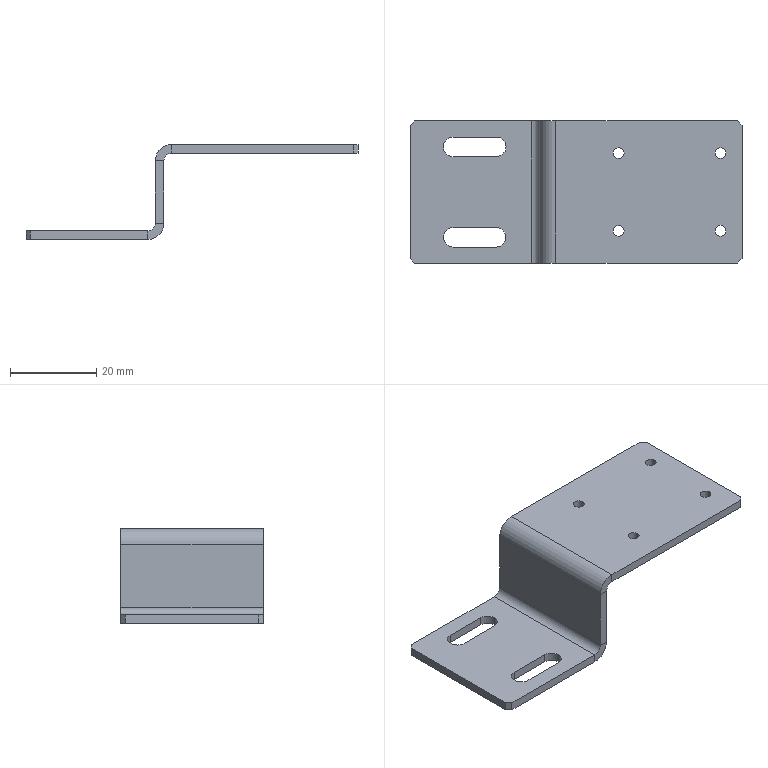Part | SolidWorks | features EdgeFlange 2, HoleWzd 2, Chamfer 1, FlatPattern 1, ICE 1, SMBaseFlange 1, SheetMetal 1 | 1 solid | 44 faces | box 77 x 33 x 22 mm | volume 5955 mm3 | plane 26 | cylinder 18 | commonest cylinder face diameters 2.5 x8 4.5 x3 4.542 x3 3.6 x2 7.6 x2
STEP:
#1=CARTESIAN_POINT('',(302.25,-22.,-2.));
#2=VERTEX_POINT('',#1);
#3=CARTESIAN_POINT('',(300.,-19.75,-2.));
#4=VERTEX_POINT('',#3);
#5=CARTESIAN_POINT('',(300.,-22.,-2.));
#6=DIRECTION('',(0.,0.,1.));
#7=DIRECTION('',(1.,0.,0.));
#8=AXIS2_PLACEMENT_3D('',#5,#6,#7);
#9=CIRCLE('',#8,2.25);
#10=EDGE_CURVE('',#2,#4,#9,.T.);
#11=ORIENTED_EDGE('',*,*,#10,.F.);
#12=CARTESIAN_POINT('',(302.25,-22.,0.));
#13=VERTEX_POINT('',#12);
#14=CARTESIAN_POINT('',(302.25,-22.,-10.));
#15=DIRECTION('',(0.,0.,1.));
#16=VECTOR('',#15,1000.);
#17=LINE('',#14,#16);
#18=EDGE_CURVE('',#2,#13,#17,.T.);
#19=ORIENTED_EDGE('',*,*,#18,.T.);
#20=CARTESIAN_POINT('',(300.,-19.75,0.));
#21=VERTEX_POINT('',#20);
#22=CARTESIAN_POINT('',(300.,-22.,0.));
#23=DIRECTION('',(0.,0.,1.));
#24=DIRECTION('',(1.,0.,0.));
#25=AXIS2_PLACEMENT_3D('',#22,#23,#24);
#26=CIRCLE('',#25,2.25);
#27=EDGE_CURVE('',#13,#21,#26,.T.);
#28=ORIENTED_EDGE('',*,*,#27,.T.);
#29=CARTESIAN_POINT('',(300.,-19.75,-10.));
#30=DIRECTION('',(0.,0.,1.));
#31=VECTOR('',#30,1000.);
#32=LINE('',#29,#31);
#33=EDGE_CURVE('',#4,#21,#32,.T.);
#34=ORIENTED_EDGE('',*,*,#33,.F.);
#35=EDGE_LOOP('',(#11,#19,#28,#34));
#36=FACE_OUTER_BOUND('',#35,.T.);
#37=CARTESIAN_POINT('',(300.,-22.,-10.));
#38=DIRECTION('',(0.,0.,1.));
#39=DIRECTION('',(1.,0.,0.));
#40=AXIS2_PLACEMENT_3D('',#37,#38,#39);
#41=CYLINDRICAL_SURFACE('',#40,2.25);
#42=ADVANCED_FACE('',(#36),#41,.F.);
#43=CARTESIAN_POINT('',(302.271,-1.,-2.));
#44=VERTEX_POINT('',#43);
#45=CARTESIAN_POINT('',(300.,1.271,-2.));
#46=VERTEX_POINT('',#45);
#47=CARTESIAN_POINT('',(300.,-1.,-2.));
#48=DIRECTION('',(0.,0.,1.));
#49=DIRECTION('',(1.,0.,0.));
#50=AXIS2_PLACEMENT_3D('',#47,#48,#49);
#51=CIRCLE('',#50,2.271);
#52=EDGE_CURVE('',#44,#46,#51,.T.);
#53=ORIENTED_EDGE('',*,*,#52,.F.);
#54=CARTESIAN_POINT('',(302.271,-1.,0.));
#55=VERTEX_POINT('',#54);
#56=CARTESIAN_POINT('',(302.271,-1.,-10.));
#57=DIRECTION('',(0.,0.,1.));
#58=VECTOR('',#57,1000.);
#59=LINE('',#56,#58);
#60=EDGE_CURVE('',#44,#55,#59,.T.);
#61=ORIENTED_EDGE('',*,*,#60,.T.);
#62=CARTESIAN_POINT('',(300.,1.271,0.));
#63=VERTEX_POINT('',#62);
#64=CARTESIAN_POINT('',(300.,-1.,0.));
#65=DIRECTION('',(0.,0.,1.));
#66=DIRECTION('',(1.,0.,0.));
#67=AXIS2_PLACEMENT_3D('',#64,#65,#66);
#68=CIRCLE('',#67,2.271);
#69=EDGE_CURVE('',#55,#63,#68,.T.);
#70=ORIENTED_EDGE('',*,*,#69,.T.);
#71=CARTESIAN_POINT('',(300.,1.271,-10.));
#72=DIRECTION('',(0.,0.,1.));
#73=VECTOR('',#72,1000.);
#74=LINE('',#71,#73);
#75=EDGE_CURVE('',#46,#63,#74,.T.);
#76=ORIENTED_EDGE('',*,*,#75,.F.);
#77=EDGE_LOOP('',(#53,#61,#70,#76));
#78=FACE_OUTER_BOUND('',#77,.T.);
#79=CARTESIAN_POINT('',(300.,-1.,-10.));
#80=DIRECTION('',(0.,0.,1.));
#81=DIRECTION('',(1.,0.,0.));
#82=AXIS2_PLACEMENT_3D('',#79,#80,#81);
#83=CYLINDRICAL_SURFACE('',#82,2.271);
#84=ADVANCED_FACE('',(#78),#83,.F.);
#85=CARTESIAN_POINT('',(329.65,-2.5,18.));
#86=VERTEX_POINT('',#85);
#87=CARTESIAN_POINT('',(327.15,-2.5,18.));
#88=VERTEX_POINT('',#87);
#89=CARTESIAN_POINT('',(328.4,-2.5,18.));
#90=DIRECTION('',(0.,0.,-1.));
#91=DIRECTION('',(-1.,0.,0.));
#92=AXIS2_PLACEMENT_3D('',#89,#90,#91);
#93=CIRCLE('',#92,1.25);
#94=EDGE_CURVE('',#86,#88,#93,.T.);
#95=ORIENTED_EDGE('',*,*,#94,.T.);
#96=CARTESIAN_POINT('',(327.15,-2.5,20.));
#97=VERTEX_POINT('',#96);
#98=CARTESIAN_POINT('',(327.15,-2.5,20.));
#99=DIRECTION('',(0.,0.,1.));
#100=VECTOR('',#99,1000.);
#101=LINE('',#98,#100);
#102=EDGE_CURVE('',#88,#97,#101,.T.);
#103=ORIENTED_EDGE('',*,*,#102,.T.);
#104=CARTESIAN_POINT('',(329.65,-2.5,20.));
#105=VERTEX_POINT('',#104);
#106=CARTESIAN_POINT('',(328.4,-2.5,20.));
#107=DIRECTION('',(0.,0.,1.));
#108=DIRECTION('',(1.,0.,0.));
#109=AXIS2_PLACEMENT_3D('',#106,#107,#108);
#110=CIRCLE('',#109,1.25);
#111=EDGE_CURVE('',#97,#105,#110,.T.);
#112=ORIENTED_EDGE('',*,*,#111,.T.);
#113=CARTESIAN_POINT('',(329.65,-2.5,20.));
#114=DIRECTION('',(0.,0.,1.));
#115=VECTOR('',#114,1000.);
#116=LINE('',#113,#115);
#117=EDGE_CURVE('',#86,#105,#116,.T.);
#118=ORIENTED_EDGE('',*,*,#117,.F.);
#119=EDGE_LOOP('',(#95,#103,#112,#118));
#120=FACE_OUTER_BOUND('',#119,.T.);
#121=CARTESIAN_POINT('',(328.4,-2.5,20.));
#122=DIRECTION('',(0.,0.,1.));
#123=DIRECTION('',(1.,0.,0.));
#124=AXIS2_PLACEMENT_3D('',#121,#122,#123);
#125=CYLINDRICAL_SURFACE('',#124,1.25);
#126=ADVANCED_FACE('',(#120),#125,.F.);
#127=CARTESIAN_POINT('',(329.65,-20.5,18.));
#128=VERTEX_POINT('',#127);
#129=CARTESIAN_POINT('',(327.15,-20.5,18.));
#130=VERTEX_POINT('',#129);
#131=CARTESIAN_POINT('',(328.4,-20.5,18.));
#132=DIRECTION('',(0.,0.,-1.));
#133=DIRECTION('',(-1.,0.,0.));
#134=AXIS2_PLACEMENT_3D('',#131,#132,#133);
#135=CIRCLE('',#134,1.25);
#136=EDGE_CURVE('',#128,#130,#135,.T.);
#137=ORIENTED_EDGE('',*,*,#136,.T.);
#138=CARTESIAN_POINT('',(327.15,-20.5,20.));
#139=VERTEX_POINT('',#138);
#140=CARTESIAN_POINT('',(327.15,-20.5,20.));
#141=DIRECTION('',(0.,0.,1.));
#142=VECTOR('',#141,1000.);
#143=LINE('',#140,#142);
#144=EDGE_CURVE('',#130,#139,#143,.T.);
#145=ORIENTED_EDGE('',*,*,#144,.T.);
#146=CARTESIAN_POINT('',(329.65,-20.5,20.));
#147=VERTEX_POINT('',#146);
#148=CARTESIAN_POINT('',(328.4,-20.5,20.));
#149=DIRECTION('',(0.,0.,1.));
#150=DIRECTION('',(1.,0.,0.));
#151=AXIS2_PLACEMENT_3D('',#148,#149,#150);
#152=CIRCLE('',#151,1.25);
#153=EDGE_CURVE('',#139,#147,#152,.T.);
#154=ORIENTED_EDGE('',*,*,#153,.T.);
#155=CARTESIAN_POINT('',(329.65,-20.5,20.));
#156=DIRECTION('',(0.,0.,1.));
#157=VECTOR('',#156,1000.);
#158=LINE('',#155,#157);
#159=EDGE_CURVE('',#128,#147,#158,.T.);
#160=ORIENTED_EDGE('',*,*,#159,.F.);
#161=EDGE_LOOP('',(#137,#145,#154,#160));
#162=FACE_OUTER_BOUND('',#161,.T.);
#163=CARTESIAN_POINT('',(328.4,-20.5,20.));
#164=DIRECTION('',(0.,0.,1.));
#165=DIRECTION('',(1.,0.,0.));
#166=AXIS2_PLACEMENT_3D('',#163,#164,#165);
#167=CYLINDRICAL_SURFACE('',#166,1.25);
#168=ADVANCED_FACE('',(#162),#167,.F.);
#169=CARTESIAN_POINT('',(353.25,-20.5,18.));
#170=VERTEX_POINT('',#169);
#171=CARTESIAN_POINT('',(350.75,-20.5,18.));
#172=VERTEX_POINT('',#171);
#173=CARTESIAN_POINT('',(352.,-20.5,18.));
#174=DIRECTION('',(0.,0.,-1.));
#175=DIRECTION('',(-1.,0.,0.));
#176=AXIS2_PLACEMENT_3D('',#173,#174,#175);
#177=CIRCLE('',#176,1.25);
#178=EDGE_CURVE('',#170,#172,#177,.T.);
#179=ORIENTED_EDGE('',*,*,#178,.T.);
#180=CARTESIAN_POINT('',(350.75,-20.5,20.));
#181=VERTEX_POINT('',#180);
#182=CARTESIAN_POINT('',(350.75,-20.5,20.));
#183=DIRECTION('',(0.,0.,1.));
#184=VECTOR('',#183,1000.);
#185=LINE('',#182,#184);
#186=EDGE_CURVE('',#172,#181,#185,.T.);
#187=ORIENTED_EDGE('',*,*,#186,.T.);
#188=CARTESIAN_POINT('',(353.25,-20.5,20.));
#189=VERTEX_POINT('',#188);
#190=CARTESIAN_POINT('',(352.,-20.5,20.));
#191=DIRECTION('',(0.,0.,1.));
#192=DIRECTION('',(1.,0.,0.));
#193=AXIS2_PLACEMENT_3D('',#190,#191,#192);
#194=CIRCLE('',#193,1.25);
#195=EDGE_CURVE('',#181,#189,#194,.T.);
#196=ORIENTED_EDGE('',*,*,#195,.T.);
#197=CARTESIAN_POINT('',(353.25,-20.5,20.));
#198=DIRECTION('',(0.,0.,1.));
#199=VECTOR('',#198,1000.);
#200=LINE('',#197,#199);
#201=EDGE_CURVE('',#170,#189,#200,.T.);
#202=ORIENTED_EDGE('',*,*,#201,.F.);
#203=EDGE_LOOP('',(#179,#187,#196,#202));
#204=FACE_OUTER_BOUND('',#203,.T.);
#205=CARTESIAN_POINT('',(352.,-20.5,20.));
#206=DIRECTION('',(0.,0.,1.));
#207=DIRECTION('',(1.,0.,0.));
#208=AXIS2_PLACEMENT_3D('',#205,#206,#207);
#209=CYLINDRICAL_SURFACE('',#208,1.25);
#210=ADVANCED_FACE('',(#204),#209,.F.);
#211=CARTESIAN_POINT('',(353.25,-2.5,18.));
#212=VERTEX_POINT('',#211);
#213=CARTESIAN_POINT('',(350.75,-2.5,18.));
#214=VERTEX_POINT('',#213);
#215=CARTESIAN_POINT('',(352.,-2.5,18.));
#216=DIRECTION('',(0.,0.,-1.));
#217=DIRECTION('',(-1.,0.,0.));
#218=AXIS2_PLACEMENT_3D('',#215,#216,#217);
#219=CIRCLE('',#218,1.25);
#220=EDGE_CURVE('',#212,#214,#219,.T.);
#221=ORIENTED_EDGE('',*,*,#220,.T.);
#222=CARTESIAN_POINT('',(350.75,-2.5,20.));
#223=VERTEX_POINT('',#222);
#224=CARTESIAN_POINT('',(350.75,-2.5,20.));
#225=DIRECTION('',(0.,0.,1.));
#226=VECTOR('',#225,1000.);
#227=LINE('',#224,#226);
#228=EDGE_CURVE('',#214,#223,#227,.T.);
#229=ORIENTED_EDGE('',*,*,#228,.T.);
#230=CARTESIAN_POINT('',(353.25,-2.5,20.));
#231=VERTEX_POINT('',#230);
#232=CARTESIAN_POINT('',(352.,-2.5,20.));
#233=DIRECTION('',(0.,0.,1.));
#234=DIRECTION('',(1.,0.,0.));
#235=AXIS2_PLACEMENT_3D('',#232,#233,#234);
#236=CIRCLE('',#235,1.25);
#237=EDGE_CURVE('',#223,#231,#236,.T.);
#238=ORIENTED_EDGE('',*,*,#237,.T.);
#239=CARTESIAN_POINT('',(353.25,-2.5,20.));
#240=DIRECTION('',(0.,0.,1.));
#241=VECTOR('',#240,1000.);
#242=LINE('',#239,#241);
#243=EDGE_CURVE('',#212,#231,#242,.T.);
#244=ORIENTED_EDGE('',*,*,#243,.F.);
#245=EDGE_LOOP('',(#221,#229,#238,#244));
#246=FACE_OUTER_BOUND('',#245,.T.);
#247=CARTESIAN_POINT('',(352.,-2.5,20.));
#248=DIRECTION('',(0.,0.,1.));
#249=DIRECTION('',(1.,0.,0.));
#250=AXIS2_PLACEMENT_3D('',#247,#248,#249);
#251=CYLINDRICAL_SURFACE('',#250,1.25);
#252=ADVANCED_FACE('',(#246),#251,.F.);
#253=CARTESIAN_POINT('',(312.,5.,16.2));
#254=VERTEX_POINT('',#253);
#255=CARTESIAN_POINT('',(310.,5.,16.2));
#256=VERTEX_POINT('',#255);
#257=CARTESIAN_POINT('',(312.,5.,16.2));
#258=DIRECTION('',(-1.,0.,0.));
#259=VECTOR('',#258,1000.);
#260=LINE('',#257,#259);
#261=EDGE_CURVE('',#254,#256,#260,.T.);
#262=ORIENTED_EDGE('',*,*,#261,.F.);
#263=CARTESIAN_POINT('',(312.,5.,1.8));
#264=VERTEX_POINT('',#263);
#265=CARTESIAN_POINT('',(312.,5.,18.));
#266=DIRECTION('',(0.,0.,1.));
#267=VECTOR('',#266,1000.);
#268=LINE('',#265,#267);
#269=EDGE_CURVE('',#264,#254,#268,.T.);
#270=ORIENTED_EDGE('',*,*,#269,.F.);
#271=CARTESIAN_POINT('',(310.,5.,1.8));
#272=VERTEX_POINT('',#271);
#273=CARTESIAN_POINT('',(310.,5.,1.8));
#274=DIRECTION('',(1.,0.,0.));
#275=VECTOR('',#274,1000.);
#276=LINE('',#273,#275);
#277=EDGE_CURVE('',#272,#264,#276,.T.);
#278=ORIENTED_EDGE('',*,*,#277,.F.);
#279=CARTESIAN_POINT('',(310.,5.,18.));
#280=DIRECTION('',(0.,0.,1.));
#281=VECTOR('',#280,1000.);
#282=LINE('',#279,#281);
#283=EDGE_CURVE('',#272,#256,#282,.T.);
#284=ORIENTED_EDGE('',*,*,#283,.T.);
#285=EDGE_LOOP('',(#262,#270,#278,#284));
#286=FACE_OUTER_BOUND('',#285,.T.);
#287=CARTESIAN_POINT('',(312.,5.,18.));
#288=DIRECTION('',(0.,-1.,0.));
#289=DIRECTION('',(0.,0.,-1.));
#290=AXIS2_PLACEMENT_3D('',#287,#288,#289);
#291=PLANE('',#290);
#292=ADVANCED_FACE('',(#286),#291,.F.);
#293=CARTESIAN_POINT('',(312.,-28.,16.2));
#294=VERTEX_POINT('',#293);
#295=CARTESIAN_POINT('',(310.,-28.,16.2));
#296=VERTEX_POINT('',#295);
#297=CARTESIAN_POINT('',(312.,-28.,16.2));
#298=DIRECTION('',(-1.,0.,0.));
#299=VECTOR('',#298,1000.);
#300=LINE('',#297,#299);
#301=EDGE_CURVE('',#294,#296,#300,.T.);
#302=ORIENTED_EDGE('',*,*,#301,.T.);
#303=CARTESIAN_POINT('',(310.,-28.,1.8));
#304=VERTEX_POINT('',#303);
#305=CARTESIAN_POINT('',(310.,-28.,0.));
#306=DIRECTION('',(0.,0.,-1.));
#307=VECTOR('',#306,1000.);
#308=LINE('',#305,#307);
#309=EDGE_CURVE('',#296,#304,#308,.T.);
#310=ORIENTED_EDGE('',*,*,#309,.T.);
#311=CARTESIAN_POINT('',(312.,-28.,1.8));
#312=VERTEX_POINT('',#311);
#313=CARTESIAN_POINT('',(310.,-28.,1.8));
#314=DIRECTION('',(1.,0.,0.));
#315=VECTOR('',#314,1000.);
#316=LINE('',#313,#315);
#317=EDGE_CURVE('',#304,#312,#316,.T.);
#318=ORIENTED_EDGE('',*,*,#317,.T.);
#319=CARTESIAN_POINT('',(312.,-28.,0.));
#320=DIRECTION('',(0.,0.,-1.));
#321=VECTOR('',#320,1000.);
#322=LINE('',#319,#321);
#323=EDGE_CURVE('',#294,#312,#322,.T.);
#324=ORIENTED_EDGE('',*,*,#323,.F.);
#325=EDGE_LOOP('',(#302,#310,#318,#324));
#326=FACE_OUTER_BOUND('',#325,.T.);
#327=CARTESIAN_POINT('',(312.,-28.,0.));
#328=DIRECTION('',(0.,1.,0.));
#329=DIRECTION('',(0.,0.,1.));
#330=AXIS2_PLACEMENT_3D('',#327,#328,#329);
#331=PLANE('',#330);
#332=ADVANCED_FACE('',(#326),#331,.F.);
#333=CARTESIAN_POINT('',(312.,-28.,16.2));
#334=DIRECTION('',(0.,1.,0.));
#335=VECTOR('',#334,1000.);
#336=LINE('',#333,#335);
#337=EDGE_CURVE('',#294,#254,#336,.T.);
#338=ORIENTED_EDGE('',*,*,#337,.F.);
#339=ORIENTED_EDGE('',*,*,#323,.T.);
#340=CARTESIAN_POINT('',(312.,0.,1.8));
#341=DIRECTION('',(0.,-1.,0.));
#342=VECTOR('',#341,1000.);
#343=LINE('',#340,#342);
#344=EDGE_CURVE('',#264,#312,#343,.T.);
#345=ORIENTED_EDGE('',*,*,#344,.F.);
#346=ORIENTED_EDGE('',*,*,#269,.T.);
#347=EDGE_LOOP('',(#338,#339,#345,#346));
#348=FACE_OUTER_BOUND('',#347,.T.);
#349=CARTESIAN_POINT('',(312.,0.,0.));
#350=DIRECTION('',(-1.,0.,0.));
#351=DIRECTION('',(0.,0.,1.));
#352=AXIS2_PLACEMENT_3D('',#349,#350,#351);
#353=PLANE('',#352);
#354=ADVANCED_FACE('',(#348),#353,.F.);
#355=ORIENTED_EDGE('',*,*,#309,.F.);
#356=CARTESIAN_POINT('',(310.,-28.,16.2));
#357=DIRECTION('',(0.,1.,0.));
#358=VECTOR('',#357,1000.);
#359=LINE('',#356,#358);
#360=EDGE_CURVE('',#296,#256,#359,.T.);
#361=ORIENTED_EDGE('',*,*,#360,.T.);
#362=ORIENTED_EDGE('',*,*,#283,.F.);
#363=CARTESIAN_POINT('',(310.,-28.,1.8));
#364=DIRECTION('',(0.,1.,0.));
#365=VECTOR('',#364,1000.);
#366=LINE('',#363,#365);
#367=EDGE_CURVE('',#304,#272,#366,.T.);
#368=ORIENTED_EDGE('',*,*,#367,.F.);
#369=EDGE_LOOP('',(#355,#361,#362,#368));
#370=FACE_OUTER_BOUND('',#369,.T.);
#371=CARTESIAN_POINT('',(310.,0.,0.));
#372=DIRECTION('',(-1.,0.,0.));
#373=DIRECTION('',(0.,0.,1.));
#374=AXIS2_PLACEMENT_3D('',#371,#372,#373);
#375=PLANE('',#374);
#376=ADVANCED_FACE('',(#370),#375,.T.);
#377=CARTESIAN_POINT('',(308.2,5.,-2.));
#378=VERTEX_POINT('',#377);
#379=CARTESIAN_POINT('',(281.,5.,-2.));
#380=VERTEX_POINT('',#379);
#381=CARTESIAN_POINT('',(280.,5.,-2.));
#382=DIRECTION('',(-1.,0.,0.));
#383=VECTOR('',#382,1000.);
#384=LINE('',#381,#383);
#385=EDGE_CURVE('',#378,#380,#384,.T.);
#386=ORIENTED_EDGE('',*,*,#385,.T.);
#387=CARTESIAN_POINT('',(281.,5.,0.));
#388=VERTEX_POINT('',#387);
#389=CARTESIAN_POINT('',(281.,5.,-2.));
#390=DIRECTION('',(0.,0.,1.));
#391=VECTOR('',#390,1000.);
#392=LINE('',#389,#391);
#393=EDGE_CURVE('',#380,#388,#392,.T.);
#394=ORIENTED_EDGE('',*,*,#393,.T.);
#395=CARTESIAN_POINT('',(308.2,5.,0.));
#396=VERTEX_POINT('',#395);
#397=CARTESIAN_POINT('',(280.,5.,0.));
#398=DIRECTION('',(-1.,0.,0.));
#399=VECTOR('',#398,1000.);
#400=LINE('',#397,#399);
#401=EDGE_CURVE('',#396,#388,#400,.T.);
#402=ORIENTED_EDGE('',*,*,#401,.F.);
#403=CARTESIAN_POINT('',(308.2,5.,0.));
#404=DIRECTION('',(0.,0.,-1.));
#405=VECTOR('',#404,1000.);
#406=LINE('',#403,#405);
#407=EDGE_CURVE('',#396,#378,#406,.T.);
#408=ORIENTED_EDGE('',*,*,#407,.T.);
#409=EDGE_LOOP('',(#386,#394,#402,#408));
#410=FACE_OUTER_BOUND('',#409,.T.);
#411=CARTESIAN_POINT('',(280.,5.,-2.));
#412=DIRECTION('',(0.,1.,0.));
#413=DIRECTION('',(0.,0.,1.));
#414=AXIS2_PLACEMENT_3D('',#411,#412,#413);
#415=PLANE('',#414);
#416=ADVANCED_FACE('',(#410),#415,.T.);
#417=CARTESIAN_POINT('',(290.,1.271,-2.));
#418=VERTEX_POINT('',#417);
#419=CARTESIAN_POINT('',(0.,1.271,-2.));
#420=DIRECTION('',(-1.,0.,0.));
#421=VECTOR('',#420,1000.);
#422=LINE('',#419,#421);
#423=EDGE_CURVE('',#46,#418,#422,.T.);
#424=ORIENTED_EDGE('',*,*,#423,.T.);
#425=CARTESIAN_POINT('',(290.,-3.271,-2.));
#426=VERTEX_POINT('',#425);
#427=CARTESIAN_POINT('',(290.,-1.,-2.));
#428=DIRECTION('',(0.,0.,1.));
#429=DIRECTION('',(1.,0.,0.));
#430=AXIS2_PLACEMENT_3D('',#427,#428,#429);
#431=CIRCLE('',#430,2.271);
#432=EDGE_CURVE('',#418,#426,#431,.T.);
#433=ORIENTED_EDGE('',*,*,#432,.T.);
#434=CARTESIAN_POINT('',(300.,-3.271,-2.));
#435=VERTEX_POINT('',#434);
#436=CARTESIAN_POINT('',(0.,-3.271,-2.));
#437=DIRECTION('',(1.,0.,0.));
#438=VECTOR('',#437,1000.);
#439=LINE('',#436,#438);
#440=EDGE_CURVE('',#426,#435,#439,.T.);
#441=ORIENTED_EDGE('',*,*,#440,.T.);
#442=CARTESIAN_POINT('',(300.,-1.,-2.));
#443=DIRECTION('',(0.,0.,1.));
#444=DIRECTION('',(1.,0.,0.));
#445=AXIS2_PLACEMENT_3D('',#442,#443,#444);
#446=CIRCLE('',#445,2.271);
#447=EDGE_CURVE('',#435,#44,#446,.T.);
#448=ORIENTED_EDGE('',*,*,#447,.T.);
#449=ORIENTED_EDGE('',*,*,#52,.T.);
#450=EDGE_LOOP('',(#424,#433,#441,#448,#449));
#451=FACE_BOUND('',#450,.T.);
#452=CARTESIAN_POINT('',(290.,-19.75,-2.));
#453=VERTEX_POINT('',#452);
#454=CARTESIAN_POINT('',(0.,-19.75,-2.));
#455=DIRECTION('',(-1.,0.,0.));
#456=VECTOR('',#455,1000.);
#457=LINE('',#454,#456);
#458=EDGE_CURVE('',#4,#453,#457,.T.);
#459=ORIENTED_EDGE('',*,*,#458,.T.);
#460=CARTESIAN_POINT('',(290.,-24.25,-2.));
#461=VERTEX_POINT('',#460);
#462=CARTESIAN_POINT('',(290.,-22.,-2.));
#463=DIRECTION('',(0.,0.,1.));
#464=DIRECTION('',(1.,0.,0.));
#465=AXIS2_PLACEMENT_3D('',#462,#463,#464);
#466=CIRCLE('',#465,2.25);
#467=EDGE_CURVE('',#453,#461,#466,.T.);
#468=ORIENTED_EDGE('',*,*,#467,.T.);
#469=CARTESIAN_POINT('',(300.,-24.25,-2.));
#470=VERTEX_POINT('',#469);
#471=CARTESIAN_POINT('',(0.,-24.25,-2.));
#472=DIRECTION('',(1.,0.,0.));
#473=VECTOR('',#472,1000.);
#474=LINE('',#471,#473);
#475=EDGE_CURVE('',#461,#470,#474,.T.);
#476=ORIENTED_EDGE('',*,*,#475,.T.);
#477=CARTESIAN_POINT('',(300.,-22.,-2.));
#478=DIRECTION('',(0.,0.,1.));
#479=DIRECTION('',(1.,0.,0.));
#480=AXIS2_PLACEMENT_3D('',#477,#478,#479);
#481=CIRCLE('',#480,2.25);
#482=EDGE_CURVE('',#470,#2,#481,.T.);
#483=ORIENTED_EDGE('',*,*,#482,.T.);
#484=ORIENTED_EDGE('',*,*,#10,.T.);
#485=EDGE_LOOP('',(#459,#468,#476,#483,#484));
#486=FACE_BOUND('',#485,.T.);
#487=CARTESIAN_POINT('',(281.,-28.,-2.));
#488=VERTEX_POINT('',#487);
#489=CARTESIAN_POINT('',(308.2,-28.,-2.));
#490=VERTEX_POINT('',#489);
#491=CARTESIAN_POINT('',(280.,-28.,-2.));
#492=DIRECTION('',(1.,0.,0.));
#493=VECTOR('',#492,1000.);
#494=LINE('',#491,#493);
#495=EDGE_CURVE('',#488,#490,#494,.T.);
#496=ORIENTED_EDGE('',*,*,#495,.F.);
#497=CARTESIAN_POINT('',(280.,-27.,-2.));
#498=VERTEX_POINT('',#497);
#499=CARTESIAN_POINT('',(280.,-27.,-2.));
#500=DIRECTION('',(-0.7071,0.7071,0.));
#501=VECTOR('',#500,1000.);
#502=LINE('',#499,#501);
#503=EDGE_CURVE('',#488,#498,#502,.T.);
#504=ORIENTED_EDGE('',*,*,#503,.T.);
#505=CARTESIAN_POINT('',(280.,4.,-2.));
#506=VERTEX_POINT('',#505);
#507=CARTESIAN_POINT('',(280.,5.,-2.));
#508=DIRECTION('',(0.,-1.,0.));
#509=VECTOR('',#508,1000.);
#510=LINE('',#507,#509);
#511=EDGE_CURVE('',#506,#498,#510,.T.);
#512=ORIENTED_EDGE('',*,*,#511,.F.);
#513=CARTESIAN_POINT('',(281.,5.,-2.));
#514=DIRECTION('',(0.7071,0.7071,0.));
#515=VECTOR('',#514,1000.);
#516=LINE('',#513,#515);
#517=EDGE_CURVE('',#506,#380,#516,.T.);
#518=ORIENTED_EDGE('',*,*,#517,.T.);
#519=ORIENTED_EDGE('',*,*,#385,.F.);
#520=CARTESIAN_POINT('',(308.2,5.,-2.));
#521=DIRECTION('',(0.,-1.,0.));
#522=VECTOR('',#521,1000.);
#523=LINE('',#520,#522);
#524=EDGE_CURVE('',#378,#490,#523,.T.);
#525=ORIENTED_EDGE('',*,*,#524,.T.);
#526=EDGE_LOOP('',(#496,#504,#512,#518,#519,#525));
#527=FACE_OUTER_BOUND('',#526,.T.);
#528=CARTESIAN_POINT('',(0.,0.,-2.));
#529=DIRECTION('',(0.,0.,1.));
#530=DIRECTION('',(1.,0.,0.));
#531=AXIS2_PLACEMENT_3D('',#528,#529,#530);
#532=PLANE('',#531);
#533=ADVANCED_FACE('',(#451,#486,#527),#532,.F.);
#534=CARTESIAN_POINT('',(290.,-19.75,0.));
#535=VERTEX_POINT('',#534);
#536=CARTESIAN_POINT('',(290.,-19.75,0.));
#537=DIRECTION('',(-1.,0.,0.));
#538=VECTOR('',#537,1000.);
#539=LINE('',#536,#538);
#540=EDGE_CURVE('',#21,#535,#539,.T.);
#541=ORIENTED_EDGE('',*,*,#540,.F.);
#542=ORIENTED_EDGE('',*,*,#27,.F.);
#543=CARTESIAN_POINT('',(300.,-24.25,0.));
#544=VERTEX_POINT('',#543);
#545=CARTESIAN_POINT('',(300.,-22.,0.));
#546=DIRECTION('',(0.,0.,1.));
#547=DIRECTION('',(1.,0.,0.));
#548=AXIS2_PLACEMENT_3D('',#545,#546,#547);
#549=CIRCLE('',#548,2.25);
#550=EDGE_CURVE('',#544,#13,#549,.T.);
#551=ORIENTED_EDGE('',*,*,#550,.F.);
#552=CARTESIAN_POINT('',(290.,-24.25,0.));
#553=VERTEX_POINT('',#552);
#554=CARTESIAN_POINT('',(290.,-24.25,0.));
#555=DIRECTION('',(1.,0.,0.));
#556=VECTOR('',#555,1000.);
#557=LINE('',#554,#556);
#558=EDGE_CURVE('',#553,#544,#557,.T.);
#559=ORIENTED_EDGE('',*,*,#558,.F.);
#560=CARTESIAN_POINT('',(290.,-22.,0.));
#561=DIRECTION('',(0.,0.,1.));
#562=DIRECTION('',(1.,0.,0.));
#563=AXIS2_PLACEMENT_3D('',#560,#561,#562);
#564=CIRCLE('',#563,2.25);
#565=EDGE_CURVE('',#535,#553,#564,.T.);
#566=ORIENTED_EDGE('',*,*,#565,.F.);
#567=EDGE_LOOP('',(#541,#542,#551,#559,#566));
#568=FACE_BOUND('',#567,.T.);
#569=CARTESIAN_POINT('',(290.,1.271,0.));
#570=VERTEX_POINT('',#569);
#571=CARTESIAN_POINT('',(290.,-3.271,0.));
#572=VERTEX_POINT('',#571);
#573=CARTESIAN_POINT('',(290.,-1.,0.));
#574=DIRECTION('',(0.,0.,1.));
#575=DIRECTION('',(1.,0.,0.));
#576=AXIS2_PLACEMENT_3D('',#573,#574,#575);
#577=CIRCLE('',#576,2.271);
#578=EDGE_CURVE('',#570,#572,#577,.T.);
#579=ORIENTED_EDGE('',*,*,#578,.F.);
#580=CARTESIAN_POINT('',(290.,1.271,0.));
#581=DIRECTION('',(-1.,0.,0.));
#582=VECTOR('',#581,1000.);
#583=LINE('',#580,#582);
#584=EDGE_CURVE('',#63,#570,#583,.T.);
#585=ORIENTED_EDGE('',*,*,#584,.F.);
#586=ORIENTED_EDGE('',*,*,#69,.F.);
#587=CARTESIAN_POINT('',(300.,-3.271,0.));
#588=VERTEX_POINT('',#587);
#589=CARTESIAN_POINT('',(300.,-1.,0.));
#590=DIRECTION('',(0.,0.,1.));
#591=DIRECTION('',(1.,0.,0.));
#592=AXIS2_PLACEMENT_3D('',#589,#590,#591);
#593=CIRCLE('',#592,2.271);
#594=EDGE_CURVE('',#588,#55,#593,.T.);
#595=ORIENTED_EDGE('',*,*,#594,.F.);
#596=CARTESIAN_POINT('',(290.,-3.271,0.));
#597=DIRECTION('',(1.,0.,0.));
#598=VECTOR('',#597,1000.);
#599=LINE('',#596,#598);
#600=EDGE_CURVE('',#572,#588,#599,.T.);
#601=ORIENTED_EDGE('',*,*,#600,.F.);
#602=EDGE_LOOP('',(#579,#585,#586,#595,#601));
#603=FACE_BOUND('',#602,.T.);
#604=CARTESIAN_POINT('',(280.,4.,0.));
#605=VERTEX_POINT('',#604);
#606=CARTESIAN_POINT('',(280.,-27.,0.));
#607=VERTEX_POINT('',#606);
#608=CARTESIAN_POINT('',(280.,5.,0.));
#609=DIRECTION('',(0.,-1.,0.));
#610=VECTOR('',#609,1000.);
#611=LINE('',#608,#610);
#612=EDGE_CURVE('',#605,#607,#611,.T.);
#613=ORIENTED_EDGE('',*,*,#612,.T.);
#614=CARTESIAN_POINT('',(281.,-28.,0.));
#615=VERTEX_POINT('',#614);
#616=CARTESIAN_POINT('',(126.5,126.5,0.));
#617=DIRECTION('',(0.7071,-0.7071,0.));
#618=VECTOR('',#617,1000.);
#619=LINE('',#616,#618);
#620=EDGE_CURVE('',#607,#615,#619,.T.);
#621=ORIENTED_EDGE('',*,*,#620,.T.);
#622=CARTESIAN_POINT('',(308.2,-28.,0.));
#623=VERTEX_POINT('',#622);
#624=CARTESIAN_POINT('',(280.,-28.,0.));
#625=DIRECTION('',(1.,0.,0.));
#626=VECTOR('',#625,1000.);
#627=LINE('',#624,#626);
#628=EDGE_CURVE('',#615,#623,#627,.T.);
#629=ORIENTED_EDGE('',*,*,#628,.T.);
#630=CARTESIAN_POINT('',(308.2,5.,0.));
#631=DIRECTION('',(0.,-1.,0.));
#632=VECTOR('',#631,1000.);
#633=LINE('',#630,#632);
#634=EDGE_CURVE('',#396,#623,#633,.T.);
#635=ORIENTED_EDGE('',*,*,#634,.F.);
#636=ORIENTED_EDGE('',*,*,#401,.T.);
#637=CARTESIAN_POINT('',(138.,-138.,0.));
#638=DIRECTION('',(-0.7071,-0.7071,0.));
#639=VECTOR('',#638,1000.);
#640=LINE('',#637,#639);
#641=EDGE_CURVE('',#388,#605,#640,.T.);
#642=ORIENTED_EDGE('',*,*,#641,.T.);
#643=EDGE_LOOP('',(#613,#621,#629,#635,#636,#642));
#644=FACE_OUTER_BOUND('',#643,.T.);
#645=CARTESIAN_POINT('',(0.,0.,0.));
#646=DIRECTION('',(0.,0.,1.));
#647=DIRECTION('',(1.,0.,0.));
#648=AXIS2_PLACEMENT_3D('',#645,#646,#647);
#649=PLANE('',#648);
#650=ADVANCED_FACE('',(#568,#603,#644),#649,.T.);
#651=ORIENTED_EDGE('',*,*,#511,.T.);
#652=CARTESIAN_POINT('',(280.,-27.,-2.));
#653=DIRECTION('',(0.,0.,1.));
#654=VECTOR('',#653,1000.);
#655=LINE('',#652,#654);
#656=EDGE_CURVE('',#498,#607,#655,.T.);
#657=ORIENTED_EDGE('',*,*,#656,.T.);
#658=ORIENTED_EDGE('',*,*,#612,.F.);
#659=CARTESIAN_POINT('',(280.,4.,-2.));
#660=DIRECTION('',(0.,0.,-1.));
#661=VECTOR('',#660,1000.);
#662=LINE('',#659,#661);
#663=EDGE_CURVE('',#605,#506,#662,.T.);
#664=ORIENTED_EDGE('',*,*,#663,.T.);
#665=EDGE_LOOP('',(#651,#657,#658,#664));
#666=FACE_OUTER_BOUND('',#665,.T.);
#667=CARTESIAN_POINT('',(280.,5.,-2.));
#668=DIRECTION('',(-1.,0.,0.));
#669=DIRECTION('',(0.,0.,1.));
#670=AXIS2_PLACEMENT_3D('',#667,#668,#669);
#671=PLANE('',#670);
#672=ADVANCED_FACE('',(#666),#671,.T.);
#673=ORIENTED_EDGE('',*,*,#628,.F.);
#674=CARTESIAN_POINT('',(281.,-28.,-2.));
#675=DIRECTION('',(0.,0.,-1.));
#676=VECTOR('',#675,1000.);
#677=LINE('',#674,#676);
#678=EDGE_CURVE('',#615,#488,#677,.T.);
#679=ORIENTED_EDGE('',*,*,#678,.T.);
#680=ORIENTED_EDGE('',*,*,#495,.T.);
#681=CARTESIAN_POINT('',(308.2,-28.,0.));
#682=DIRECTION('',(0.,0.,-1.));
#683=VECTOR('',#682,1000.);
#684=LINE('',#681,#683);
#685=EDGE_CURVE('',#623,#490,#684,.T.);
#686=ORIENTED_EDGE('',*,*,#685,.F.);
#687=EDGE_LOOP('',(#673,#679,#680,#686));
#688=FACE_OUTER_BOUND('',#687,.T.);
#689=CARTESIAN_POINT('',(280.,-28.,-2.));
#690=DIRECTION('',(0.,-1.,0.));
#691=DIRECTION('',(0.,0.,-1.));
#692=AXIS2_PLACEMENT_3D('',#689,#690,#691);
#693=PLANE('',#692);
#694=ADVANCED_FACE('',(#688),#693,.T.);
#695=ORIENTED_EDGE('',*,*,#317,.F.);
#696=CARTESIAN_POINT('',(308.2,-28.,1.8));
#697=DIRECTION('',(0.,-1.,0.));
#698=DIRECTION('',(0.,0.,1.));
#699=AXIS2_PLACEMENT_3D('',#696,#697,#698);
#700=CIRCLE('',#699,1.8);
#701=EDGE_CURVE('',#623,#304,#700,.T.);
#702=ORIENTED_EDGE('',*,*,#701,.F.);
#703=ORIENTED_EDGE('',*,*,#685,.T.);
#704=CARTESIAN_POINT('',(308.2,-28.,1.8));
#705=DIRECTION('',(0.,-1.,0.));
#706=DIRECTION('',(0.,0.,1.));
#707=AXIS2_PLACEMENT_3D('',#704,#705,#706);
#708=CIRCLE('',#707,3.8);
#709=EDGE_CURVE('',#490,#312,#708,.T.);
#710=ORIENTED_EDGE('',*,*,#709,.T.);
#711=EDGE_LOOP('',(#695,#702,#703,#710));
#712=FACE_OUTER_BOUND('',#711,.T.);
#713=CARTESIAN_POINT('',(308.2,-28.,1.8));
#714=DIRECTION('',(0.,-1.,0.));
#715=DIRECTION('',(0.,0.,-1.));
#716=AXIS2_PLACEMENT_3D('',#713,#714,#715);
#717=PLANE('',#716);
#718=ADVANCED_FACE('',(#712),#717,.T.);
#719=CARTESIAN_POINT('',(308.2,5.,1.8));
#720=DIRECTION('',(0.,1.,0.));
#721=DIRECTION('',(0.,0.,1.));
#722=AXIS2_PLACEMENT_3D('',#719,#720,#721);
#723=CIRCLE('',#722,1.8);
#724=EDGE_CURVE('',#272,#396,#723,.T.);
#725=ORIENTED_EDGE('',*,*,#724,.F.);
#726=ORIENTED_EDGE('',*,*,#277,.T.);
#727=CARTESIAN_POINT('',(308.2,5.,1.8));
#728=DIRECTION('',(0.,1.,0.));
#729=DIRECTION('',(0.,0.,1.));
#730=AXIS2_PLACEMENT_3D('',#727,#728,#729);
#731=CIRCLE('',#730,3.8);
#732=EDGE_CURVE('',#264,#378,#731,.T.);
#733=ORIENTED_EDGE('',*,*,#732,.T.);
#734=ORIENTED_EDGE('',*,*,#407,.F.);
#735=EDGE_LOOP('',(#725,#726,#733,#734));
#736=FACE_OUTER_BOUND('',#735,.T.);
#737=CARTESIAN_POINT('',(308.2,5.,1.8));
#738=DIRECTION('',(0.,-1.,0.));
#739=DIRECTION('',(0.,0.,-1.));
#740=AXIS2_PLACEMENT_3D('',#737,#738,#739);
#741=PLANE('',#740);
#742=ADVANCED_FACE('',(#736),#741,.F.);
#743=ORIENTED_EDGE('',*,*,#524,.F.);
#744=ORIENTED_EDGE('',*,*,#732,.F.);
#745=ORIENTED_EDGE('',*,*,#344,.T.);
#746=ORIENTED_EDGE('',*,*,#709,.F.);
#747=EDGE_LOOP('',(#743,#744,#745,#746));
#748=FACE_OUTER_BOUND('',#747,.T.);
#749=CARTESIAN_POINT('',(308.2,5.,1.8));
#750=DIRECTION('',(0.,1.,0.));
#751=DIRECTION('',(1.,0.,0.));
#752=AXIS2_PLACEMENT_3D('',#749,#750,#751);
#753=CYLINDRICAL_SURFACE('',#752,3.8);
#754=ADVANCED_FACE('',(#748),#753,.T.);
#755=ORIENTED_EDGE('',*,*,#634,.T.);
#756=ORIENTED_EDGE('',*,*,#701,.T.);
#757=ORIENTED_EDGE('',*,*,#367,.T.);
#758=ORIENTED_EDGE('',*,*,#724,.T.);
#759=EDGE_LOOP('',(#755,#756,#757,#758));
#760=FACE_OUTER_BOUND('',#759,.T.);
#761=CARTESIAN_POINT('',(308.2,5.,1.8));
#762=DIRECTION('',(0.,1.,0.));
#763=DIRECTION('',(1.,0.,0.));
#764=AXIS2_PLACEMENT_3D('',#761,#762,#763);
#765=CYLINDRICAL_SURFACE('',#764,1.8);
#766=ADVANCED_FACE('',(#760),#765,.F.);
#767=CARTESIAN_POINT('',(313.8,5.,18.));
#768=VERTEX_POINT('',#767);
#769=CARTESIAN_POINT('',(313.8,5.,20.));
#770=VERTEX_POINT('',#769);
#771=CARTESIAN_POINT('',(313.8,5.,18.));
#772=DIRECTION('',(0.,0.,1.));
#773=VECTOR('',#772,1000.);
#774=LINE('',#771,#773);
#775=EDGE_CURVE('',#768,#770,#774,.T.);
#776=ORIENTED_EDGE('',*,*,#775,.F.);
#777=CARTESIAN_POINT('',(313.8,5.,16.2));
#778=DIRECTION('',(0.,1.,0.));
#779=DIRECTION('',(0.,0.,-1.));
#780=AXIS2_PLACEMENT_3D('',#777,#778,#779);
#781=CIRCLE('',#780,1.8);
#782=EDGE_CURVE('',#254,#768,#781,.T.);
#783=ORIENTED_EDGE('',*,*,#782,.F.);
#784=ORIENTED_EDGE('',*,*,#261,.T.);
#785=CARTESIAN_POINT('',(313.8,5.,16.2));
#786=DIRECTION('',(0.,1.,0.));
#787=DIRECTION('',(0.,0.,-1.));
#788=AXIS2_PLACEMENT_3D('',#785,#786,#787);
#789=CIRCLE('',#788,3.8);
#790=EDGE_CURVE('',#256,#770,#789,.T.);
#791=ORIENTED_EDGE('',*,*,#790,.T.);
#792=EDGE_LOOP('',(#776,#783,#784,#791));
#793=FACE_OUTER_BOUND('',#792,.T.);
#794=CARTESIAN_POINT('',(313.8,5.,16.2));
#795=DIRECTION('',(0.,1.,0.));
#796=DIRECTION('',(0.,0.,1.));
#797=AXIS2_PLACEMENT_3D('',#794,#795,#796);
#798=PLANE('',#797);
#799=ADVANCED_FACE('',(#793),#798,.T.);
#800=CARTESIAN_POINT('',(313.8,-28.,18.));
#801=VERTEX_POINT('',#800);
#802=CARTESIAN_POINT('',(313.8,-28.,16.2));
#803=DIRECTION('',(0.,-1.,0.));
#804=DIRECTION('',(0.,0.,-1.));
#805=AXIS2_PLACEMENT_3D('',#802,#803,#804);
#806=CIRCLE('',#805,1.8);
#807=EDGE_CURVE('',#801,#294,#806,.T.);
#808=ORIENTED_EDGE('',*,*,#807,.F.);
#809=CARTESIAN_POINT('',(313.8,-28.,20.));
#810=VERTEX_POINT('',#809);
#811=CARTESIAN_POINT('',(313.8,-28.,18.));
#812=DIRECTION('',(0.,0.,1.));
#813=VECTOR('',#812,1000.);
#814=LINE('',#811,#813);
#815=EDGE_CURVE('',#801,#810,#814,.T.);
#816=ORIENTED_EDGE('',*,*,#815,.T.);
#817=CARTESIAN_POINT('',(313.8,-28.,16.2));
#818=DIRECTION('',(0.,-1.,0.));
#819=DIRECTION('',(0.,0.,-1.));
#820=AXIS2_PLACEMENT_3D('',#817,#818,#819);
#821=CIRCLE('',#820,3.8);
#822=EDGE_CURVE('',#810,#296,#821,.T.);
#823=ORIENTED_EDGE('',*,*,#822,.T.);
#824=ORIENTED_EDGE('',*,*,#301,.F.);
#825=EDGE_LOOP('',(#808,#816,#823,#824));
#826=FACE_OUTER_BOUND('',#825,.T.);
#827=CARTESIAN_POINT('',(313.8,-28.,16.2));
#828=DIRECTION('',(0.,1.,0.));
#829=DIRECTION('',(0.,0.,1.));
#830=AXIS2_PLACEMENT_3D('',#827,#828,#829);
#831=PLANE('',#830);
#832=ADVANCED_FACE('',(#826),#831,.F.);
#833=ORIENTED_EDGE('',*,*,#360,.F.);
#834=ORIENTED_EDGE('',*,*,#822,.F.);
#835=CARTESIAN_POINT('',(313.8,0.,20.));
#836=DIRECTION('',(0.,1.,0.));
#837=VECTOR('',#836,1000.);
#838=LINE('',#835,#837);
#839=EDGE_CURVE('',#810,#770,#838,.T.);
#840=ORIENTED_EDGE('',*,*,#839,.T.);
#841=ORIENTED_EDGE('',*,*,#790,.F.);
#842=EDGE_LOOP('',(#833,#834,#840,#841));
#843=FACE_OUTER_BOUND('',#842,.T.);
#844=CARTESIAN_POINT('',(313.8,-28.,16.2));
#845=DIRECTION('',(0.,-1.,0.));
#846=DIRECTION('',(0.,0.,1.));
#847=AXIS2_PLACEMENT_3D('',#844,#845,#846);
#848=CYLINDRICAL_SURFACE('',#847,3.8);
#849=ADVANCED_FACE('',(#843),#848,.T.);
#850=ORIENTED_EDGE('',*,*,#337,.T.);
#851=ORIENTED_EDGE('',*,*,#782,.T.);
#852=CARTESIAN_POINT('',(313.8,5.,18.));
#853=DIRECTION('',(0.,-1.,0.));
#854=VECTOR('',#853,1000.);
#855=LINE('',#852,#854);
#856=EDGE_CURVE('',#768,#801,#855,.T.);
#857=ORIENTED_EDGE('',*,*,#856,.T.);
#858=ORIENTED_EDGE('',*,*,#807,.T.);
#859=EDGE_LOOP('',(#850,#851,#857,#858));
#860=FACE_OUTER_BOUND('',#859,.T.);
#861=CARTESIAN_POINT('',(313.8,-28.,16.2));
#862=DIRECTION('',(0.,-1.,0.));
#863=DIRECTION('',(0.,0.,1.));
#864=AXIS2_PLACEMENT_3D('',#861,#862,#863);
#865=CYLINDRICAL_SURFACE('',#864,1.8);
#866=ADVANCED_FACE('',(#860),#865,.F.);
#867=CARTESIAN_POINT('',(356.,-28.,18.));
#868=VERTEX_POINT('',#867);
#869=CARTESIAN_POINT('',(357.,-28.,18.));
#870=DIRECTION('',(1.,0.,0.));
#871=VECTOR('',#870,1000.);
#872=LINE('',#869,#871);
#873=EDGE_CURVE('',#801,#868,#872,.T.);
#874=ORIENTED_EDGE('',*,*,#873,.T.);
#875=CARTESIAN_POINT('',(356.,-28.,20.));
#876=VERTEX_POINT('',#875);
#877=CARTESIAN_POINT('',(356.,-28.,20.));
#878=DIRECTION('',(0.,0.,1.));
#879=VECTOR('',#878,1000.);
#880=LINE('',#877,#879);
#881=EDGE_CURVE('',#868,#876,#880,.T.);
#882=ORIENTED_EDGE('',*,*,#881,.T.);
#883=CARTESIAN_POINT('',(357.,-28.,20.));
#884=DIRECTION('',(1.,0.,0.));
#885=VECTOR('',#884,1000.);
#886=LINE('',#883,#885);
#887=EDGE_CURVE('',#810,#876,#886,.T.);
#888=ORIENTED_EDGE('',*,*,#887,.F.);
#889=ORIENTED_EDGE('',*,*,#815,.F.);
#890=EDGE_LOOP('',(#874,#882,#888,#889));
#891=FACE_OUTER_BOUND('',#890,.T.);
#892=CARTESIAN_POINT('',(357.,-28.,20.));
#893=DIRECTION('',(0.,1.,0.));
#894=DIRECTION('',(0.,0.,1.));
#895=AXIS2_PLACEMENT_3D('',#892,#893,#894);
#896=PLANE('',#895);
#897=ADVANCED_FACE('',(#891),#896,.F.);
#898=CARTESIAN_POINT('',(356.,5.,20.));
#899=VERTEX_POINT('',#898);
#900=CARTESIAN_POINT('',(312.,5.,20.));
#901=DIRECTION('',(-1.,0.,0.));
#902=VECTOR('',#901,1000.);
#903=LINE('',#900,#902);
#904=EDGE_CURVE('',#899,#770,#903,.T.);
#905=ORIENTED_EDGE('',*,*,#904,.F.);
#906=CARTESIAN_POINT('',(356.,5.,18.));
#907=VERTEX_POINT('',#906);
#908=CARTESIAN_POINT('',(356.,5.,20.));
#909=DIRECTION('',(0.,0.,-1.));
#910=VECTOR('',#909,1000.);
#911=LINE('',#908,#910);
#912=EDGE_CURVE('',#899,#907,#911,.T.);
#913=ORIENTED_EDGE('',*,*,#912,.T.);
#914=CARTESIAN_POINT('',(312.,5.,18.));
#915=DIRECTION('',(-1.,0.,0.));
#916=VECTOR('',#915,1000.);
#917=LINE('',#914,#916);
#918=EDGE_CURVE('',#907,#768,#917,.T.);
#919=ORIENTED_EDGE('',*,*,#918,.T.);
#920=ORIENTED_EDGE('',*,*,#775,.T.);
#921=EDGE_LOOP('',(#905,#913,#919,#920));
#922=FACE_OUTER_BOUND('',#921,.T.);
#923=CARTESIAN_POINT('',(312.,5.,20.));
#924=DIRECTION('',(0.,-1.,0.));
#925=DIRECTION('',(0.,0.,-1.));
#926=AXIS2_PLACEMENT_3D('',#923,#924,#925);
#927=PLANE('',#926);
#928=ADVANCED_FACE('',(#922),#927,.F.);
#929=CARTESIAN_POINT('',(328.4,-2.5,20.));
#930=DIRECTION('',(0.,0.,1.));
#931=DIRECTION('',(1.,0.,0.));
#932=AXIS2_PLACEMENT_3D('',#929,#930,#931);
#933=CIRCLE('',#932,1.25);
#934=EDGE_CURVE('',#105,#97,#933,.T.);
#935=ORIENTED_EDGE('',*,*,#934,.F.);
#936=ORIENTED_EDGE('',*,*,#111,.F.);
#937=EDGE_LOOP('',(#935,#936));
#938=FACE_BOUND('',#937,.T.);
#939=CARTESIAN_POINT('',(328.4,-20.5,20.));
#940=DIRECTION('',(0.,0.,1.));
#941=DIRECTION('',(1.,0.,0.));
#942=AXIS2_PLACEMENT_3D('',#939,#940,#941);
#943=CIRCLE('',#942,1.25);
#944=EDGE_CURVE('',#147,#139,#943,.T.);
#945=ORIENTED_EDGE('',*,*,#944,.F.);
#946=ORIENTED_EDGE('',*,*,#153,.F.);
#947=EDGE_LOOP('',(#945,#946));
#948=FACE_BOUND('',#947,.T.);
#949=CARTESIAN_POINT('',(352.,-20.5,20.));
#950=DIRECTION('',(0.,0.,1.));
#951=DIRECTION('',(1.,0.,0.));
#952=AXIS2_PLACEMENT_3D('',#949,#950,#951);
#953=CIRCLE('',#952,1.25);
#954=EDGE_CURVE('',#189,#181,#953,.T.);
#955=ORIENTED_EDGE('',*,*,#954,.F.);
#956=ORIENTED_EDGE('',*,*,#195,.F.);
#957=EDGE_LOOP('',(#955,#956));
#958=FACE_BOUND('',#957,.T.);
#959=CARTESIAN_POINT('',(352.,-2.5,20.));
#960=DIRECTION('',(0.,0.,1.));
#961=DIRECTION('',(1.,0.,0.));
#962=AXIS2_PLACEMENT_3D('',#959,#960,#961);
#963=CIRCLE('',#962,1.25);
#964=EDGE_CURVE('',#231,#223,#963,.T.);
#965=ORIENTED_EDGE('',*,*,#964,.F.);
#966=ORIENTED_EDGE('',*,*,#237,.F.);
#967=EDGE_LOOP('',(#965,#966));
#968=FACE_BOUND('',#967,.T.);
#969=ORIENTED_EDGE('',*,*,#887,.T.);
#970=CARTESIAN_POINT('',(357.,-27.,20.));
#971=VERTEX_POINT('',#970);
#972=CARTESIAN_POINT('',(357.,-27.,20.));
#973=DIRECTION('',(0.7071,0.7071,0.));
#974=VECTOR('',#973,1000.);
#975=LINE('',#972,#974);
#976=EDGE_CURVE('',#876,#971,#975,.T.);
#977=ORIENTED_EDGE('',*,*,#976,.T.);
#978=CARTESIAN_POINT('',(357.,4.,20.));
#979=VERTEX_POINT('',#978);
#980=CARTESIAN_POINT('',(357.,5.,20.));
#981=DIRECTION('',(0.,1.,0.));
#982=VECTOR('',#981,1000.);
#983=LINE('',#980,#982);
#984=EDGE_CURVE('',#971,#979,#983,.T.);
#985=ORIENTED_EDGE('',*,*,#984,.T.);
#986=CARTESIAN_POINT('',(356.,5.,20.));
#987=DIRECTION('',(-0.7071,0.7071,0.));
#988=VECTOR('',#987,1000.);
#989=LINE('',#986,#988);
#990=EDGE_CURVE('',#979,#899,#989,.T.);
#991=ORIENTED_EDGE('',*,*,#990,.T.);
#992=ORIENTED_EDGE('',*,*,#904,.T.);
#993=ORIENTED_EDGE('',*,*,#839,.F.);
#994=EDGE_LOOP('',(#969,#977,#985,#991,#992,#993));
#995=FACE_OUTER_BOUND('',#994,.T.);
#996=CARTESIAN_POINT('',(0.,0.,20.));
#997=DIRECTION('',(0.,0.,-1.));
#998=DIRECTION('',(-1.,0.,0.));
#999=AXIS2_PLACEMENT_3D('',#996,#997,#998);
#1000=PLANE('',#999);
#1001=ADVANCED_FACE('',(#938,#948,#958,#968,#995),#1000,.F.);
#1002=ORIENTED_EDGE('',*,*,#94,.F.);
#1003=CARTESIAN_POINT('',(328.4,-2.5,18.));
#1004=DIRECTION('',(0.,0.,-1.));
#1005=DIRECTION('',(-1.,0.,0.));
#1006=AXIS2_PLACEMENT_3D('',#1003,#1004,#1005);
#1007=CIRCLE('',#1006,1.25);
#1008=EDGE_CURVE('',#88,#86,#1007,.T.);
#1009=ORIENTED_EDGE('',*,*,#1008,.F.);
#1010=EDGE_LOOP('',(#1002,#1009));
#1011=FACE_BOUND('',#1010,.T.);
#1012=ORIENTED_EDGE('',*,*,#136,.F.);
#1013=CARTESIAN_POINT('',(328.4,-20.5,18.));
#1014=DIRECTION('',(0.,0.,-1.));
#1015=DIRECTION('',(-1.,0.,0.));
#1016=AXIS2_PLACEMENT_3D('',#1013,#1014,#1015);
#1017=CIRCLE('',#1016,1.25);
#1018=EDGE_CURVE('',#130,#128,#1017,.T.);
#1019=ORIENTED_EDGE('',*,*,#1018,.F.);
#1020=EDGE_LOOP('',(#1012,#1019));
#1021=FACE_BOUND('',#1020,.T.);
#1022=ORIENTED_EDGE('',*,*,#178,.F.);
#1023=CARTESIAN_POINT('',(352.,-20.5,18.));
#1024=DIRECTION('',(0.,0.,-1.));
#1025=DIRECTION('',(-1.,0.,0.));
#1026=AXIS2_PLACEMENT_3D('',#1023,#1024,#1025);
#1027=CIRCLE('',#1026,1.25);
#1028=EDGE_CURVE('',#172,#170,#1027,.T.);
#1029=ORIENTED_EDGE('',*,*,#1028,.F.);
#1030=EDGE_LOOP('',(#1022,#1029));
#1031=FACE_BOUND('',#1030,.T.);
#1032=ORIENTED_EDGE('',*,*,#220,.F.);
#1033=CARTESIAN_POINT('',(352.,-2.5,18.));
#1034=DIRECTION('',(0.,0.,-1.));
#1035=DIRECTION('',(-1.,0.,0.));
#1036=AXIS2_PLACEMENT_3D('',#1033,#1034,#1035);
#1037=CIRCLE('',#1036,1.25);
#1038=EDGE_CURVE('',#214,#212,#1037,.T.);
#1039=ORIENTED_EDGE('',*,*,#1038,.F.);
#1040=EDGE_LOOP('',(#1032,#1039));
#1041=FACE_BOUND('',#1040,.T.);
#1042=CARTESIAN_POINT('',(357.,-27.,18.));
#1043=VERTEX_POINT('',#1042);
#1044=CARTESIAN_POINT('',(357.,4.,18.));
#1045=VERTEX_POINT('',#1044);
#1046=CARTESIAN_POINT('',(357.,5.,18.));
#1047=DIRECTION('',(0.,1.,0.));
#1048=VECTOR('',#1047,1000.);
#1049=LINE('',#1046,#1048);
#1050=EDGE_CURVE('',#1043,#1045,#1049,.T.);
#1051=ORIENTED_EDGE('',*,*,#1050,.F.);
#1052=CARTESIAN_POINT('',(192.,-192.,18.));
#1053=DIRECTION('',(-0.7071,-0.7071,0.));
#1054=VECTOR('',#1053,1000.);
#1055=LINE('',#1052,#1054);
#1056=EDGE_CURVE('',#1043,#868,#1055,.T.);
#1057=ORIENTED_EDGE('',*,*,#1056,.T.);
#1058=ORIENTED_EDGE('',*,*,#873,.F.);
#1059=ORIENTED_EDGE('',*,*,#856,.F.);
#1060=ORIENTED_EDGE('',*,*,#918,.F.);
#1061=CARTESIAN_POINT('',(180.5,180.5,18.));
#1062=DIRECTION('',(0.7071,-0.7071,0.));
#1063=VECTOR('',#1062,1000.);
#1064=LINE('',#1061,#1063);
#1065=EDGE_CURVE('',#907,#1045,#1064,.T.);
#1066=ORIENTED_EDGE('',*,*,#1065,.T.);
#1067=EDGE_LOOP('',(#1051,#1057,#1058,#1059,#1060,#1066));
#1068=FACE_OUTER_BOUND('',#1067,.T.);
#1069=CARTESIAN_POINT('',(0.,0.,18.));
#1070=DIRECTION('',(0.,0.,-1.));
#1071=DIRECTION('',(-1.,0.,0.));
#1072=AXIS2_PLACEMENT_3D('',#1069,#1070,#1071);
#1073=PLANE('',#1072);
#1074=ADVANCED_FACE('',(#1011,#1021,#1031,#1041,#1068),#1073,.T.);
#1075=ORIENTED_EDGE('',*,*,#984,.F.);
#1076=CARTESIAN_POINT('',(357.,-27.,20.));
#1077=DIRECTION('',(0.,0.,-1.));
#1078=VECTOR('',#1077,1000.);
#1079=LINE('',#1076,#1078);
#1080=EDGE_CURVE('',#971,#1043,#1079,.T.);
#1081=ORIENTED_EDGE('',*,*,#1080,.T.);
#1082=ORIENTED_EDGE('',*,*,#1050,.T.);
#1083=CARTESIAN_POINT('',(357.,4.,20.));
#1084=DIRECTION('',(0.,0.,1.));
#1085=VECTOR('',#1084,1000.);
#1086=LINE('',#1083,#1085);
#1087=EDGE_CURVE('',#1045,#979,#1086,.T.);
#1088=ORIENTED_EDGE('',*,*,#1087,.T.);
#1089=EDGE_LOOP('',(#1075,#1081,#1082,#1088));
#1090=FACE_OUTER_BOUND('',#1089,.T.);
#1091=CARTESIAN_POINT('',(357.,5.,20.));
#1092=DIRECTION('',(-1.,0.,0.));
#1093=DIRECTION('',(0.,0.,1.));
#1094=AXIS2_PLACEMENT_3D('',#1091,#1092,#1093);
#1095=PLANE('',#1094);
#1096=ADVANCED_FACE('',(#1090),#1095,.F.);
#1097=ORIENTED_EDGE('',*,*,#228,.F.);
#1098=ORIENTED_EDGE('',*,*,#1038,.T.);
#1099=ORIENTED_EDGE('',*,*,#243,.T.);
#1100=ORIENTED_EDGE('',*,*,#964,.T.);
#1101=EDGE_LOOP('',(#1097,#1098,#1099,#1100));
#1102=FACE_OUTER_BOUND('',#1101,.T.);
#1103=CARTESIAN_POINT('',(352.,-2.5,20.));
#1104=DIRECTION('',(0.,0.,1.));
#1105=DIRECTION('',(1.,0.,0.));
#1106=AXIS2_PLACEMENT_3D('',#1103,#1104,#1105);
#1107=CYLINDRICAL_SURFACE('',#1106,1.25);
#1108=ADVANCED_FACE('',(#1102),#1107,.F.);
#1109=ORIENTED_EDGE('',*,*,#186,.F.);
#1110=ORIENTED_EDGE('',*,*,#1028,.T.);
#1111=ORIENTED_EDGE('',*,*,#201,.T.);
#1112=ORIENTED_EDGE('',*,*,#954,.T.);
#1113=EDGE_LOOP('',(#1109,#1110,#1111,#1112));
#1114=FACE_OUTER_BOUND('',#1113,.T.);
#1115=CARTESIAN_POINT('',(352.,-20.5,20.));
#1116=DIRECTION('',(0.,0.,1.));
#1117=DIRECTION('',(1.,0.,0.));
#1118=AXIS2_PLACEMENT_3D('',#1115,#1116,#1117);
#1119=CYLINDRICAL_SURFACE('',#1118,1.25);
#1120=ADVANCED_FACE('',(#1114),#1119,.F.);
#1121=ORIENTED_EDGE('',*,*,#144,.F.);
#1122=ORIENTED_EDGE('',*,*,#1018,.T.);
#1123=ORIENTED_EDGE('',*,*,#159,.T.);
#1124=ORIENTED_EDGE('',*,*,#944,.T.);
#1125=EDGE_LOOP('',(#1121,#1122,#1123,#1124));
#1126=FACE_OUTER_BOUND('',#1125,.T.);
#1127=CARTESIAN_POINT('',(328.4,-20.5,20.));
#1128=DIRECTION('',(0.,0.,1.));
#1129=DIRECTION('',(1.,0.,0.));
#1130=AXIS2_PLACEMENT_3D('',#1127,#1128,#1129);
#1131=CYLINDRICAL_SURFACE('',#1130,1.25);
#1132=ADVANCED_FACE('',(#1126),#1131,.F.);
#1133=ORIENTED_EDGE('',*,*,#102,.F.);
#1134=ORIENTED_EDGE('',*,*,#1008,.T.);
#1135=ORIENTED_EDGE('',*,*,#117,.T.);
#1136=ORIENTED_EDGE('',*,*,#934,.T.);
#1137=EDGE_LOOP('',(#1133,#1134,#1135,#1136));
#1138=FACE_OUTER_BOUND('',#1137,.T.);
#1139=CARTESIAN_POINT('',(328.4,-2.5,20.));
#1140=DIRECTION('',(0.,0.,1.));
#1141=DIRECTION('',(1.,0.,0.));
#1142=AXIS2_PLACEMENT_3D('',#1139,#1140,#1141);
#1143=CYLINDRICAL_SURFACE('',#1142,1.25);
#1144=ADVANCED_FACE('',(#1138),#1143,.F.);
#1145=CARTESIAN_POINT('',(290.,1.271,-10.));
#1146=DIRECTION('',(0.,0.,1.));
#1147=VECTOR('',#1146,1000.);
#1148=LINE('',#1145,#1147);
#1149=EDGE_CURVE('',#418,#570,#1148,.T.);
#1150=ORIENTED_EDGE('',*,*,#1149,.T.);
#1151=ORIENTED_EDGE('',*,*,#578,.T.);
#1152=CARTESIAN_POINT('',(290.,-3.271,-10.));
#1153=DIRECTION('',(0.,0.,1.));
#1154=VECTOR('',#1153,1000.);
#1155=LINE('',#1152,#1154);
#1156=EDGE_CURVE('',#426,#572,#1155,.T.);
#1157=ORIENTED_EDGE('',*,*,#1156,.F.);
#1158=ORIENTED_EDGE('',*,*,#432,.F.);
#1159=EDGE_LOOP('',(#1150,#1151,#1157,#1158));
#1160=FACE_OUTER_BOUND('',#1159,.T.);
#1161=CARTESIAN_POINT('',(290.,-1.,-10.));
#1162=DIRECTION('',(0.,0.,1.));
#1163=DIRECTION('',(1.,0.,0.));
#1164=AXIS2_PLACEMENT_3D('',#1161,#1162,#1163);
#1165=CYLINDRICAL_SURFACE('',#1164,2.271);
#1166=ADVANCED_FACE('',(#1160),#1165,.F.);
#1167=ORIENTED_EDGE('',*,*,#75,.T.);
#1168=ORIENTED_EDGE('',*,*,#584,.T.);
#1169=ORIENTED_EDGE('',*,*,#1149,.F.);
#1170=ORIENTED_EDGE('',*,*,#423,.F.);
#1171=EDGE_LOOP('',(#1167,#1168,#1169,#1170));
#1172=FACE_OUTER_BOUND('',#1171,.T.);
#1173=CARTESIAN_POINT('',(290.,1.271,-10.));
#1174=DIRECTION('',(0.,1.,0.));
#1175=DIRECTION('',(0.,0.,1.));
#1176=AXIS2_PLACEMENT_3D('',#1173,#1174,#1175);
#1177=PLANE('',#1176);
#1178=ADVANCED_FACE('',(#1172),#1177,.F.);
#1179=ORIENTED_EDGE('',*,*,#60,.F.);
#1180=ORIENTED_EDGE('',*,*,#447,.F.);
#1181=CARTESIAN_POINT('',(300.,-3.271,-10.));
#1182=DIRECTION('',(0.,0.,1.));
#1183=VECTOR('',#1182,1000.);
#1184=LINE('',#1181,#1183);
#1185=EDGE_CURVE('',#435,#588,#1184,.T.);
#1186=ORIENTED_EDGE('',*,*,#1185,.T.);
#1187=ORIENTED_EDGE('',*,*,#594,.T.);
#1188=EDGE_LOOP('',(#1179,#1180,#1186,#1187));
#1189=FACE_OUTER_BOUND('',#1188,.T.);
#1190=CARTESIAN_POINT('',(300.,-1.,-10.));
#1191=DIRECTION('',(0.,0.,1.));
#1192=DIRECTION('',(1.,0.,0.));
#1193=AXIS2_PLACEMENT_3D('',#1190,#1191,#1192);
#1194=CYLINDRICAL_SURFACE('',#1193,2.271);
#1195=ADVANCED_FACE('',(#1189),#1194,.F.);
#1196=ORIENTED_EDGE('',*,*,#1156,.T.);
#1197=ORIENTED_EDGE('',*,*,#600,.T.);
#1198=ORIENTED_EDGE('',*,*,#1185,.F.);
#1199=ORIENTED_EDGE('',*,*,#440,.F.);
#1200=EDGE_LOOP('',(#1196,#1197,#1198,#1199));
#1201=FACE_OUTER_BOUND('',#1200,.T.);
#1202=CARTESIAN_POINT('',(290.,-3.271,-10.));
#1203=DIRECTION('',(0.,-1.,0.));
#1204=DIRECTION('',(0.,0.,-1.));
#1205=AXIS2_PLACEMENT_3D('',#1202,#1203,#1204);
#1206=PLANE('',#1205);
#1207=ADVANCED_FACE('',(#1201),#1206,.F.);
#1208=CARTESIAN_POINT('',(290.,-19.75,-10.));
#1209=DIRECTION('',(0.,0.,1.));
#1210=VECTOR('',#1209,1000.);
#1211=LINE('',#1208,#1210);
#1212=EDGE_CURVE('',#453,#535,#1211,.T.);
#1213=ORIENTED_EDGE('',*,*,#1212,.T.);
#1214=ORIENTED_EDGE('',*,*,#565,.T.);
#1215=CARTESIAN_POINT('',(290.,-24.25,-10.));
#1216=DIRECTION('',(0.,0.,1.));
#1217=VECTOR('',#1216,1000.);
#1218=LINE('',#1215,#1217);
#1219=EDGE_CURVE('',#461,#553,#1218,.T.);
#1220=ORIENTED_EDGE('',*,*,#1219,.F.);
#1221=ORIENTED_EDGE('',*,*,#467,.F.);
#1222=EDGE_LOOP('',(#1213,#1214,#1220,#1221));
#1223=FACE_OUTER_BOUND('',#1222,.T.);
#1224=CARTESIAN_POINT('',(290.,-22.,-10.));
#1225=DIRECTION('',(0.,0.,1.));
#1226=DIRECTION('',(1.,0.,0.));
#1227=AXIS2_PLACEMENT_3D('',#1224,#1225,#1226);
#1228=CYLINDRICAL_SURFACE('',#1227,2.25);
#1229=ADVANCED_FACE('',(#1223),#1228,.F.);
#1230=ORIENTED_EDGE('',*,*,#18,.F.);
#1231=ORIENTED_EDGE('',*,*,#482,.F.);
#1232=CARTESIAN_POINT('',(300.,-24.25,-10.));
#1233=DIRECTION('',(0.,0.,1.));
#1234=VECTOR('',#1233,1000.);
#1235=LINE('',#1232,#1234);
#1236=EDGE_CURVE('',#470,#544,#1235,.T.);
#1237=ORIENTED_EDGE('',*,*,#1236,.T.);
#1238=ORIENTED_EDGE('',*,*,#550,.T.);
#1239=EDGE_LOOP('',(#1230,#1231,#1237,#1238));
#1240=FACE_OUTER_BOUND('',#1239,.T.);
#1241=CARTESIAN_POINT('',(300.,-22.,-10.));
#1242=DIRECTION('',(0.,0.,1.));
#1243=DIRECTION('',(1.,0.,0.));
#1244=AXIS2_PLACEMENT_3D('',#1241,#1242,#1243);
#1245=CYLINDRICAL_SURFACE('',#1244,2.25);
#1246=ADVANCED_FACE('',(#1240),#1245,.F.);
#1247=ORIENTED_EDGE('',*,*,#33,.T.);
#1248=ORIENTED_EDGE('',*,*,#540,.T.);
#1249=ORIENTED_EDGE('',*,*,#1212,.F.);
#1250=ORIENTED_EDGE('',*,*,#458,.F.);
#1251=EDGE_LOOP('',(#1247,#1248,#1249,#1250));
#1252=FACE_OUTER_BOUND('',#1251,.T.);
#1253=CARTESIAN_POINT('',(290.,-19.75,-10.));
#1254=DIRECTION('',(0.,1.,0.));
#1255=DIRECTION('',(0.,0.,1.));
#1256=AXIS2_PLACEMENT_3D('',#1253,#1254,#1255);
#1257=PLANE('',#1256);
#1258=ADVANCED_FACE('',(#1252),#1257,.F.);
#1259=ORIENTED_EDGE('',*,*,#1219,.T.);
#1260=ORIENTED_EDGE('',*,*,#558,.T.);
#1261=ORIENTED_EDGE('',*,*,#1236,.F.);
#1262=ORIENTED_EDGE('',*,*,#475,.F.);
#1263=EDGE_LOOP('',(#1259,#1260,#1261,#1262));
#1264=FACE_OUTER_BOUND('',#1263,.T.);
#1265=CARTESIAN_POINT('',(290.,-24.25,-10.));
#1266=DIRECTION('',(0.,-1.,0.));
#1267=DIRECTION('',(0.,0.,-1.));
#1268=AXIS2_PLACEMENT_3D('',#1265,#1266,#1267);
#1269=PLANE('',#1268);
#1270=ADVANCED_FACE('',(#1264),#1269,.F.);
#1271=ORIENTED_EDGE('',*,*,#976,.F.);
#1272=ORIENTED_EDGE('',*,*,#881,.F.);
#1273=ORIENTED_EDGE('',*,*,#1056,.F.);
#1274=ORIENTED_EDGE('',*,*,#1080,.F.);
#1275=EDGE_LOOP('',(#1271,#1272,#1273,#1274));
#1276=FACE_OUTER_BOUND('',#1275,.T.);
#1277=CARTESIAN_POINT('',(357.,-27.,20.));
#1278=DIRECTION('',(-0.7071,0.7071,0.));
#1279=DIRECTION('',(0.,0.,-1.));
#1280=AXIS2_PLACEMENT_3D('',#1277,#1278,#1279);
#1281=PLANE('',#1280);
#1282=ADVANCED_FACE('',(#1276),#1281,.F.);
#1283=ORIENTED_EDGE('',*,*,#990,.F.);
#1284=ORIENTED_EDGE('',*,*,#1087,.F.);
#1285=ORIENTED_EDGE('',*,*,#1065,.F.);
#1286=ORIENTED_EDGE('',*,*,#912,.F.);
#1287=EDGE_LOOP('',(#1283,#1284,#1285,#1286));
#1288=FACE_OUTER_BOUND('',#1287,.T.);
#1289=CARTESIAN_POINT('',(356.,5.,20.));
#1290=DIRECTION('',(-0.7071,-0.7071,0.));
#1291=DIRECTION('',(0.,0.,-1.));
#1292=AXIS2_PLACEMENT_3D('',#1289,#1290,#1291);
#1293=PLANE('',#1292);
#1294=ADVANCED_FACE('',(#1288),#1293,.F.);
#1295=ORIENTED_EDGE('',*,*,#503,.F.);
#1296=ORIENTED_EDGE('',*,*,#678,.F.);
#1297=ORIENTED_EDGE('',*,*,#620,.F.);
#1298=ORIENTED_EDGE('',*,*,#656,.F.);
#1299=EDGE_LOOP('',(#1295,#1296,#1297,#1298));
#1300=FACE_OUTER_BOUND('',#1299,.T.);
#1301=CARTESIAN_POINT('',(280.,-27.,-2.));
#1302=DIRECTION('',(0.7071,0.7071,0.));
#1303=DIRECTION('',(0.,0.,1.));
#1304=AXIS2_PLACEMENT_3D('',#1301,#1302,#1303);
#1305=PLANE('',#1304);
#1306=ADVANCED_FACE('',(#1300),#1305,.F.);
#1307=ORIENTED_EDGE('',*,*,#517,.F.);
#1308=ORIENTED_EDGE('',*,*,#663,.F.);
#1309=ORIENTED_EDGE('',*,*,#641,.F.);
#1310=ORIENTED_EDGE('',*,*,#393,.F.);
#1311=EDGE_LOOP('',(#1307,#1308,#1309,#1310));
#1312=FACE_OUTER_BOUND('',#1311,.T.);
#1313=CARTESIAN_POINT('',(281.,5.,-2.));
#1314=DIRECTION('',(0.7071,-0.7071,0.));
#1315=DIRECTION('',(0.,0.,1.));
#1316=AXIS2_PLACEMENT_3D('',#1313,#1314,#1315);
#1317=PLANE('',#1316);
#1318=ADVANCED_FACE('',(#1312),#1317,.F.);
#1319=CLOSED_SHELL('',(#42,#84,#126,#168,#210,#252,#292,#332,#354,#376,#416,#533,#650,#672,#694,#718,#742,#754,#766,#799,#832,#849,#866,#897,#928,#1001,#1074,#1096,#1108,#1120,#1132,#1144,#1166,#1178,#1195,#1207,#1229,#1246,#1258,#1270,#1282,#1294,#1306,#1318));
#1320=MANIFOLD_SOLID_BREP('',#1319);
#1321=CARTESIAN_POINT('',(0.,0.,0.));
#1322=DIRECTION('',(0.,0.,1.));
#1323=DIRECTION('',(1.,0.,0.));
#1324=AXIS2_PLACEMENT_3D('',#1321,#1322,#1323);
#1325=(LENGTH_UNIT()NAMED_UNIT(*)SI_UNIT(.MILLI.,.METRE.));
#1326=UNCERTAINTY_MEASURE_WITH_UNIT(LENGTH_MEASURE(0.00001),#1325,'','');
#1327=(NAMED_UNIT(*)PLANE_ANGLE_UNIT()SI_UNIT($,.RADIAN.));
#1328=(NAMED_UNIT(*)SI_UNIT($,.STERADIAN.)SOLID_ANGLE_UNIT());
#1329=(GEOMETRIC_REPRESENTATION_CONTEXT(3)GLOBAL_UNCERTAINTY_ASSIGNED_CONTEXT((#1326))GLOBAL_UNIT_ASSIGNED_CONTEXT((#1325,#1327,#1328))REPRESENTATION_CONTEXT('',''));
#1330=ADVANCED_BREP_SHAPE_REPRESENTATION('',(#1320,#1324),#1329);